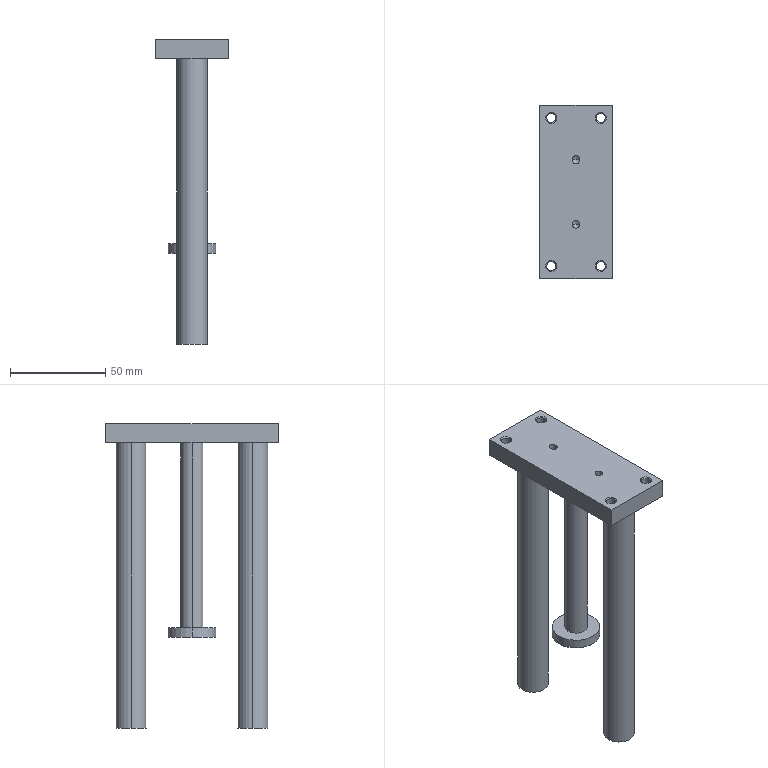Part | SolidWorks | features BaseBody 1 | 1 solid | 56 faces | box 38 x 91 x 160 mm | volume 107406 mm3 | cylinder 22 | cone 20 | plane 14 | commonest cylinder face diameters 4.917 x8 4 x6 16 x4 12 x2 25 x2